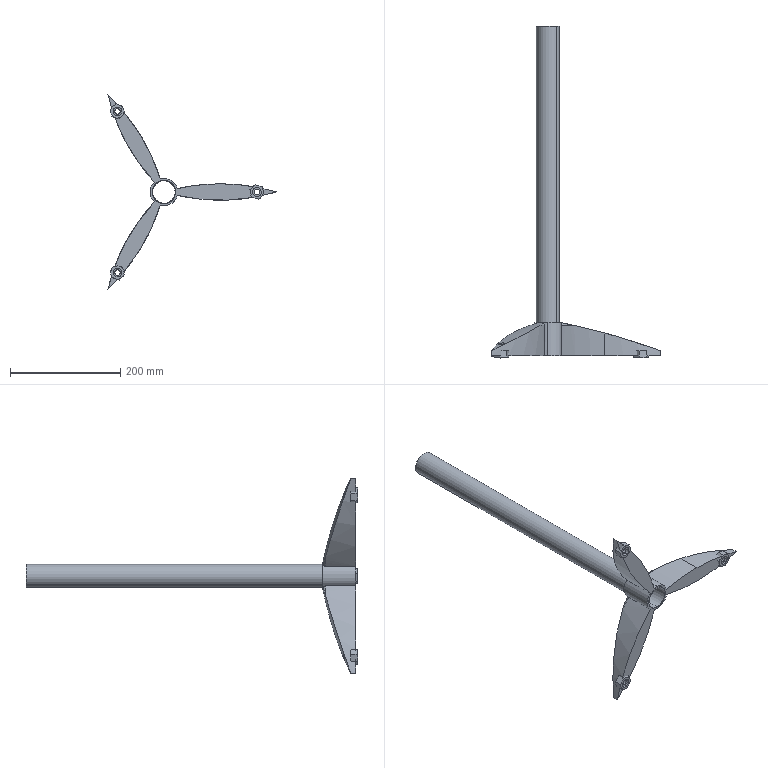Part | SolidWorks | 2 solids | 111 faces | box 305.237 x 601.627 x 352.457 mm | volume 571557 mm3 | cone 39 | cylinder 35 | plane 28 | spline 9 | commonest cylinder face diameters 16 x12 700.36 x7 10.028 x6 50 x4 40.56 x2 42.16 x2